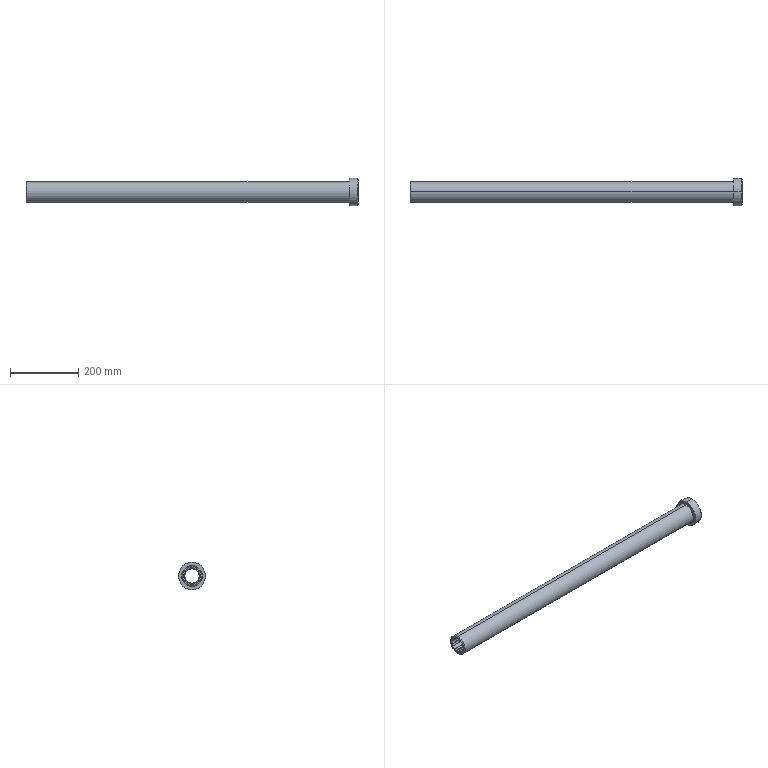Part | SolidWorks | features Chamfer 3, ICE 3, Extrusion 1, Fillet 1 | 1 solid | 65 faces | box 975 x 80 x 80 mm | volume 1427415 mm3 | plane 27 | cone 21 | cylinder 15 | torus 2 | commonest cylinder face diameters 48.475 x9 42 x2 60 x2 80 x2